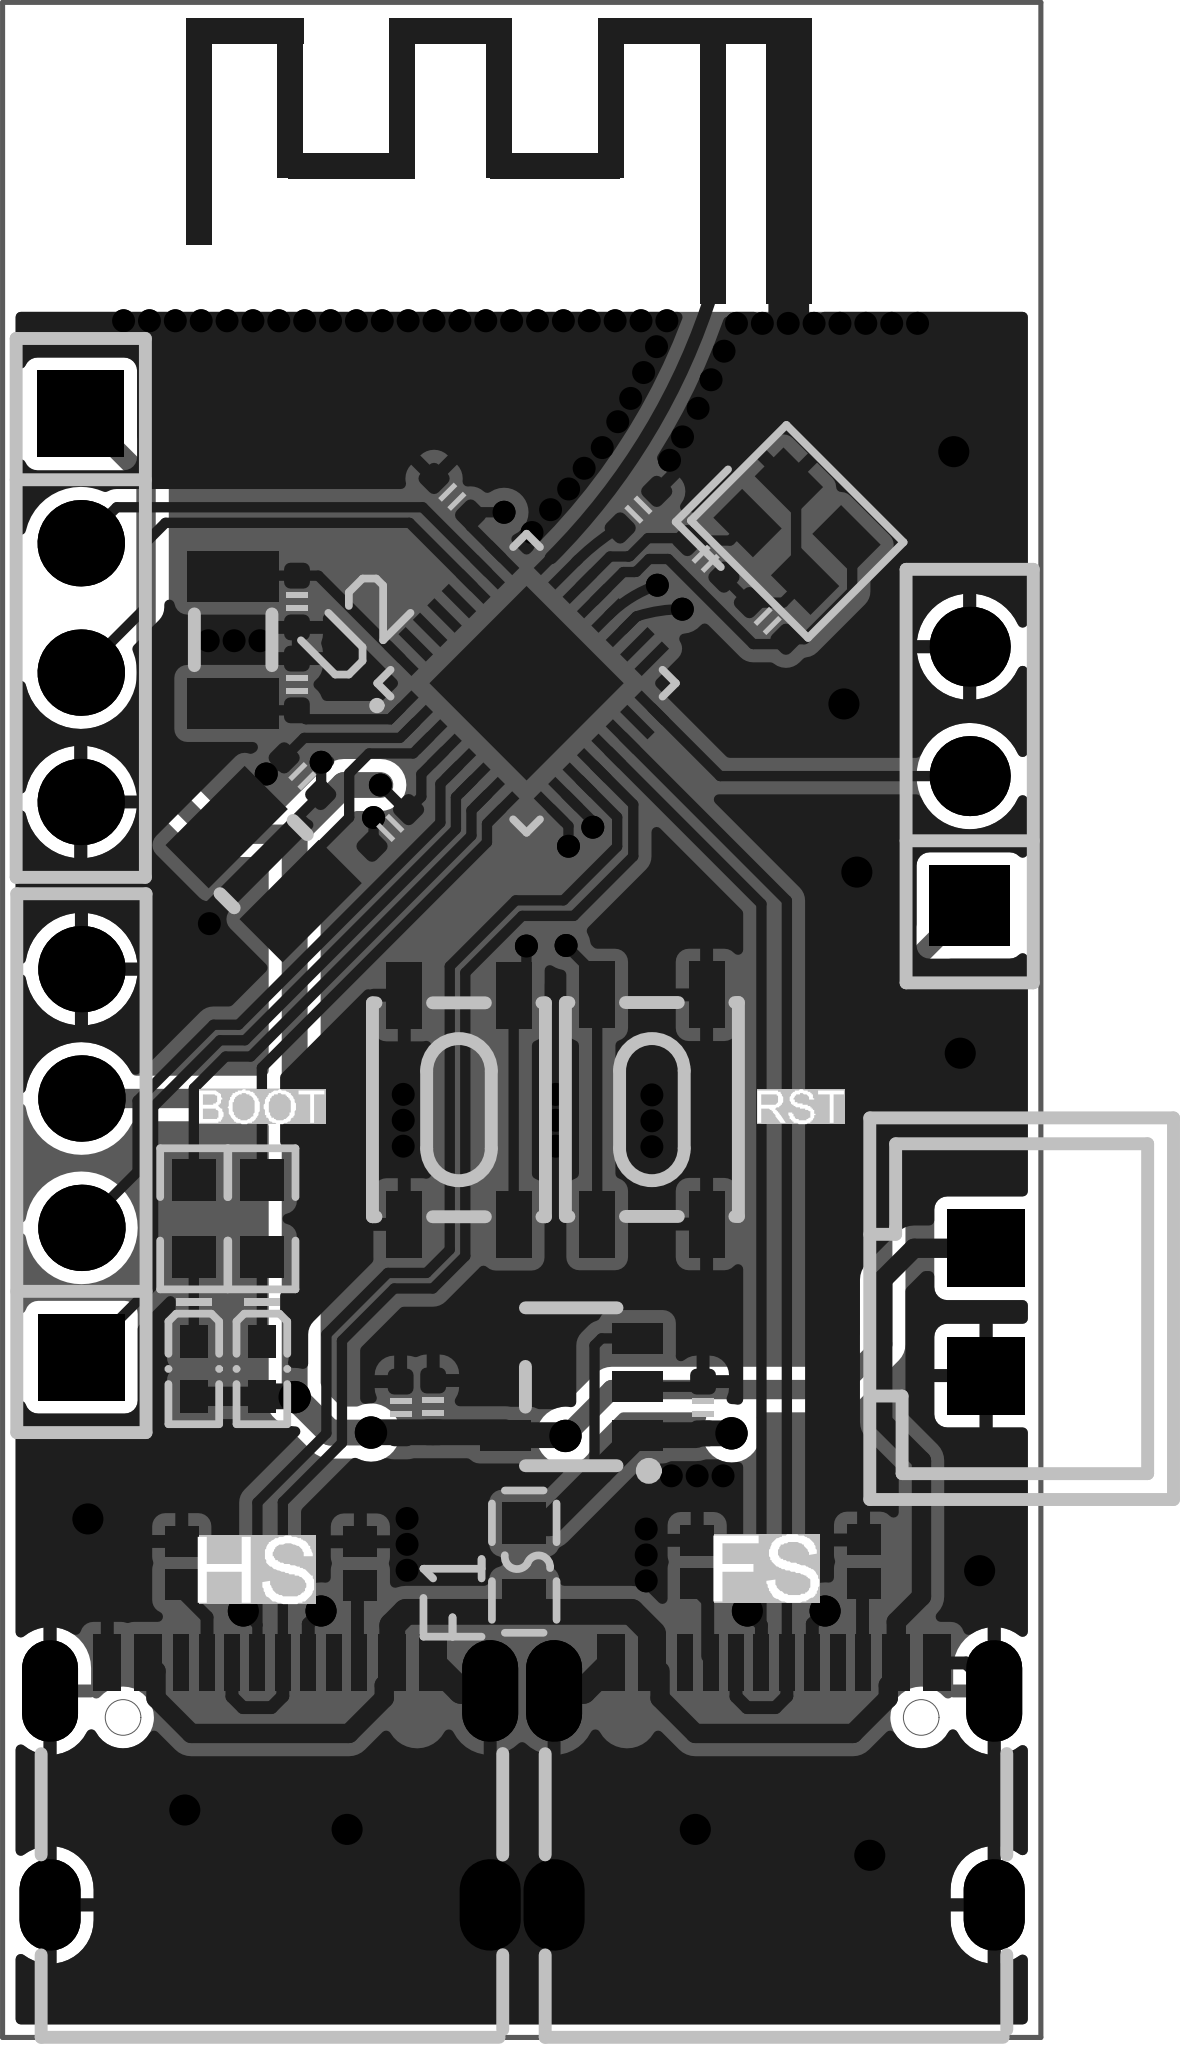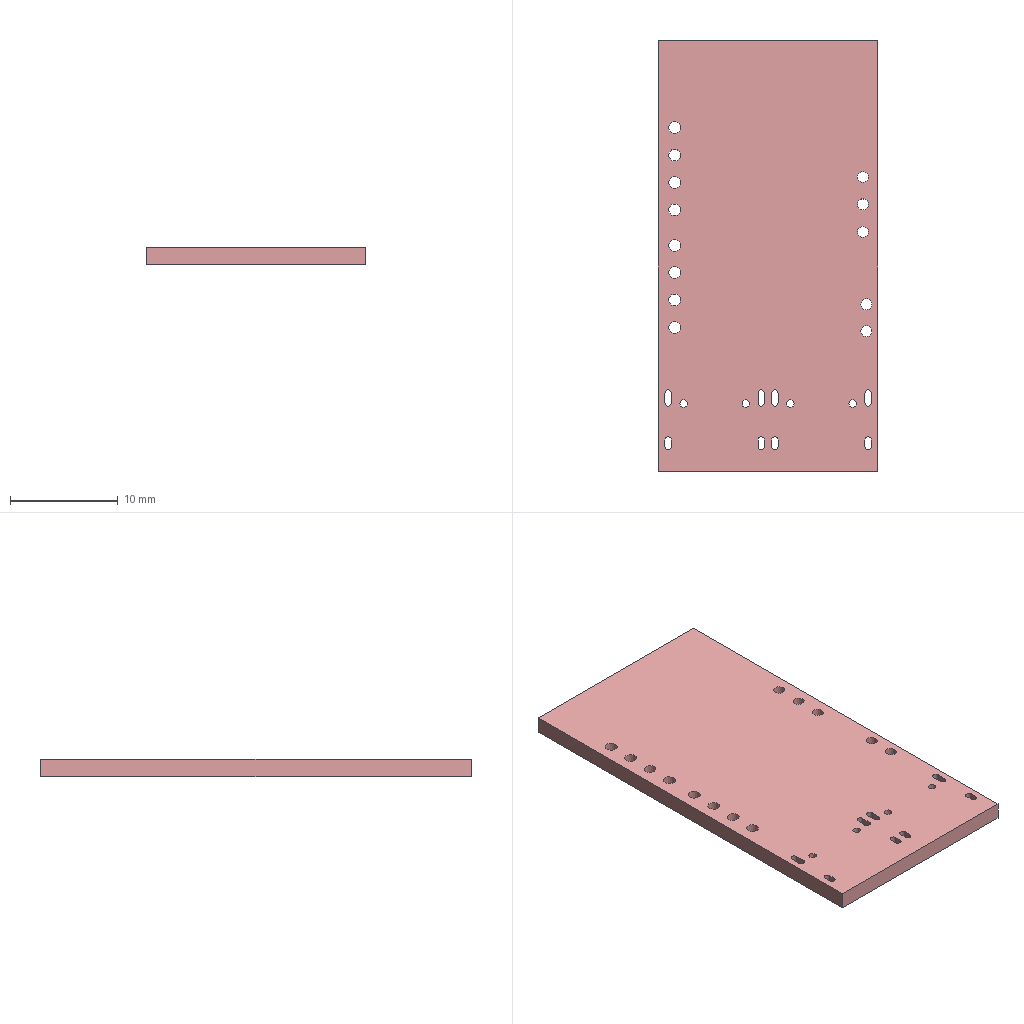Circuit board layout | Altium Designer | box 20.4 x 40 x 1.6 mm
Layer stack:
# Altium Designer layer stack of  (unit mm; dielectric type: 0 none, 1 core, 2 prepreg, 3 surface material)
index,name,kind,layer,copper_thickness_mm,dielectric_type,dielectric_thickness_mm,dielectric_material,dielectric_constant
0,Top Paste Mask Layer,other,,,,,,
1,Top Silkscreen Layer,other,,,,,,
2,Top Solder Mask Layer,dielectric,,,3,0.01,,3.3
3,Top Layer,copper,Top Layer,0.035,,,,
4,SUBSTRATE1,dielectric,,,3,1.51,FR4,4.5
5,Bottom Layer,copper,Bottom Layer,0.035,,,,
6,Bottom Solder Mask Layer,dielectric,,,3,0.01,,3.3
7,Bottom Silkscreen Layer,other,,,,,,
8,Bottom Paste Mask Layer,other,,,,,,
# drill layer pairs: low layer,high layer
drill_pair,Top Layer,Bottom Layer
Part placement:
Designator,Comment,Layer,Footprint,Center-X(mm),Center-Y(mm),Rotation
USB1,TYPE-C 16PIN 2MD(073),TopLayer,USB-C-SMD_TYPE-C-6PIN-2MD-073,87.808,88.367,0
USB2,TYPE-C 16PIN 2MD(073),TopLayer,USB-C-SMD_TYPE-C-6PIN-2MD-073,97.714,88.367,0
BOOT1,K2-1808SN-A3SW-01,TopLayer,SW-SMD_4P-L4.2-W3.3-P2.15-LS5.1,91.519,101.603,270
L2,10uH,TopLayer,IND-SMD_L2.5-W2.0,87.681,106.426,135
X2,32.768kHz,TopLayer,FC-135R_L3.2-W1.5,87.082,110.831,90
E1,,TopLayer,ANT-F-1-2.4G-1.6mmFR4,97.259,117.736,0
R10,5.1kΩ,TopLayer,R0402,99.471,92.731,270
LED1,SZYY0402B,TopLayer,LED0402-RD_BLUE,86.308,96.515,270
R14,1kΩ,TopLayer,R0603,86.308,99.462,270
C8,100nF,TopLayer,0402电容（极简封装）,91.013,95.779,270
U4,RT9013-33GB,TopLayer,SOT-23-5_L3.0-W1.7-P0.95-LS2.8-BR,93.726,96.164,0
U5,32MHz,TopLayer,CRYSTAL-SMD_4P-L2.0-W1.6-BL-2,98.163,112.963,315
F1,BSMD0603-050-6V,TopLayer,F0603,92.802,92.731,90
C23,1uF,TopLayer,0402电容（极简封装）,96.317,95.758,270
C24,1uF,TopLayer,0402电容（极简封装）,90.373,95.758,270
C1,100nF,TopLayer,0402电容（极简封装）,91.389,113.64,135
C2,470nF,TopLayer,0402电容（极简封装）,95.047,113.386,45
C3,2.2uF,TopLayer,0402电容（极简封装）,90.17,107.137,225
C6,4.7uF,TopLayer,0402电容（极简封装）,88.443,108.153,135
C19,NC,TopLayer,0402电容（极简封装）,96.368,112.42,135
C20,NC,TopLayer,0402电容（极简封装）,88.334,109.954,90
C21,NC,TopLayer,0402电容（极简封装）,88.336,111.582,270
C22,NC,TopLayer,0402电容（极简封装）,97.587,111.201,315
LED2,SZYY0402B,TopLayer,LED0402-RD_BLUE,87.646,96.515,270
RST1,K2-1808SN-A3SW-01,TopLayer,SW-SMD_4P-L4.2-W3.3-P2.15-LS5.1,95.311,101.609,90
R11,5.1kΩ,TopLayer,R0402,96.201,92.724,270
R12,5.1kΩ,TopLayer,R0402,89.582,92.696,270
R13,5.1kΩ,TopLayer,R0402,86.072,92.702,270
R15,1kΩ,TopLayer,R0603,87.646,99.462,270
U2,CH584F,TopLayer,QFN-32_L4.0-W4.0-P0.40-TL-EP2.7,92.848,109.978,45
H1,,TopLayer,HDR-TH_4P-P2.54-V-F,84.087,111.457,270
H2,,TopLayer,HDR-TH_3P-P2.54-V-F,101.557,108.154,90
P1,XH2.54 through-hole socket-2P,TopLayer,CONN-TH_XH2.54-2P,101.879,97.634,270
H3,,TopLayer,HDR-TH_4P-P2.54-V-F,84.099,100.555,90
Pad and via stacks:
# Altium Designer via and pad stacks of  (unit mm). Each distinct definition once, with the count of objects using it.
# via: kind,start_layer,end_layer,hole_mm,diameter_mm,mode(0 simple;1 top-mid-bottom;2 full stack),diameter_per_layer,count,example_net
# pad: kind,layer,hole_mm,hole_type(0 round;1 square;2 slot),plating,top_size,top_shape(1 round;2 rect;3 octagon;9 rounded rect),mid_size,bottom_size,mode,footprint,size_per_layer,count,example
pad,Top Layer,0,0,plated,0.55x1.1,2,0.55x1.1,0.55x1.1,0,USB-C-SMD_TYPE-C-6PIN-2MD-073,,8,USB1.1
pad,Top Layer,0,0,plated,0.3x1.1,2,0.3x1.1,0.3x1.1,0,USB-C-SMD_TYPE-C-6PIN-2MD-073,,16,USB1.3
pad,Top Layer,0,0,plated,0.7x1.3,2,0.7x1.3,0.7x1.3,0,SW-SMD_4P-L4.2-W3.3-P2.15-LS5.1,,8,BOOT1.1
pad,Top Layer,0,0,plated,1.2x2.2,2,1.2x2.2,1.2x2.2,0,IND-SMD_L2.5-W2.0,,2,L2.1
pad,Top Layer,0,0,plated,1.8x1,2,1.8x1,1.8x1,0,FC-135R_L3.2-W1.5,,2,X2.1
pad,Top Layer,0,0,plated,0.6x0.8,2,0.6x0.8,0.6x0.8,0,ANT-F-1-2.4G-1.6mmFR4,,1,E1.0
pad,Top Layer,0,0,plated,0.6x0.4,2,0.6x0.4,0.6x0.4,0,ANT-F-1-2.4G-1.6mmFR4,,1,E1.1
pad,Top Layer,0,0,plated,0.6x0.65,2,0.6x0.65,0.6x0.65,0,R0402,,8,R10.1
pad,Top Layer,0,0,plated,0.6365x0.54,2,0.6365x0.54,0.6365x0.54,0,LED0402-RD_BLUE,,4,LED1.2
pad,Top Layer,0,0,plated,0.8065x0.864,2,0.8065x0.864,0.8065x0.864,0,R0603,,4,R14.2
pad,Top Layer,0,0,plated,0.254x0.254,1,0.254x0.254,0.254x0.254,0,0402\u00B5\u00E7\u00C8\u00DD\u00A3\u00A8\u00BC\u00AB\u00BC\u00F2\u00B7\u00E2\u00D7\u00B0\u00A3\u00A9,,22,C8.2
pad,Top Layer,0,0,plated,1x0.6,2,1x0.6,1x0.6,0,SOT-23-5_L3.0-W1.7-P0.95-LS2.8-BR,,5,U4.5
pad,Top Layer,0,0,plated,1.1x0.8,2,1.1x0.8,1.1x0.8,0,CRYSTAL-SMD_4P-L2.0-W1.6-BL-2,,4,U5.1
pad,Top Layer,0,0,plated,0.8065x0.864,2,0.8065x0.864,0.8065x0.864,0,F0603,,2,F1.2
pad,Top Layer,0,0,plated,0.76x0.2,2,0.76x0.2,0.76x0.2,0,QFN-32_L4.0-W4.0-P0.40-TL-EP2.7,,16,U2.1
pad,Top Layer,0,0,plated,0.2x0.76,2,0.2x0.76,0.2x0.76,0,QFN-32_L4.0-W4.0-P0.40-TL-EP2.7,,16,U2.9
pad,Top Layer,0,0,plated,2.7x2.7,2,2.7x2.7,2.7x2.7,0,QFN-32_L4.0-W4.0-P0.40-TL-EP2.7,,1,U2.33
pad,Multi-Layer,0.6,2,plated,1.1x2,1,1.1x2,1.1x2,0,USB-C-SMD_TYPE-C-6PIN-2MD-073,,4,USB1.13
pad,Multi-Layer,0.6,2,plated,1.2x1.8,1,1.2x1.8,1.2x1.8,0,USB-C-SMD_TYPE-C-6PIN-2MD-073,,4,USB1.13
pad,Multi-Layer,1.1,0,plated,1.7x1.7,2,1.7x1.7,1.7x1.7,0,HDR-TH_4P-P2.54-V-F,,2,H1.1
pad,Multi-Layer,1.1,0,plated,1.7x1.7,1,1.7x1.7,1.7x1.7,0,HDR-TH_4P-P2.54-V-F,,6,H1.2
pad,Multi-Layer,1.02,0,plated,1.575x1.575,1,1.575x1.575,1.575x1.575,0,HDR-TH_3P-P2.54-V-F,,2,H2.3
pad,Multi-Layer,1.02,0,plated,1.575x1.575,2,1.575x1.575,1.575x1.575,0,HDR-TH_3P-P2.54-V-F,,1,H2.1
pad,Multi-Layer,1,2,plated,1.524x1.524,2,1.524x1.524,1.524x1.524,0,CONN-TH_XH2.54-2P,,2,P1.1
via,Top Layer,Bottom Layer,0.3048,0.61,0,,14,PB11
via,Top Layer,Bottom Layer,0.3048,0.45,0,,102,BOOT
via,Top Layer,Bottom Layer,0.4572,0.635,0,,4,+5V
Copper pours:
name,layer,net,type(0 solid;1 hatched;2 none)
Bottom Layer-GND,Bottom Layer,GND,0
Top Layer-GND,Top Layer,GND,0
Design rules, without the lines most boards share:
# Altium Designer design rules of  (exported by Altium Designer, unit mm)
# columns: name | kind | enabled | priority | scope1 | scope2 | descriptor | typed fields (field=value)
copperThickness1oz | 0 | enabled | 4 | All | All | Clearance Constraint (Gap=0mil) (All),(All) | gap=0
otherClearance | 52 | enabled | 1 | All | All | Hole To Hole Clearance (Gap=0mil) (All),(All) | gap=0
viaSize | 11 | enabled | 1 | All | All | Routing Via (MinHoleWidth=0.394mil) (MaxHoleWidth=472.441mil) (PreferredHoleWidth=0.394mil) (MinWidth=0.394mil) (MaxWidth=472.441mil) (PreferedWidth=0.394mil) (All) | via_min_hole=0.01 via_max_hole=12 via_preferred_diameter=0.01 via_preferred_hole=0.01